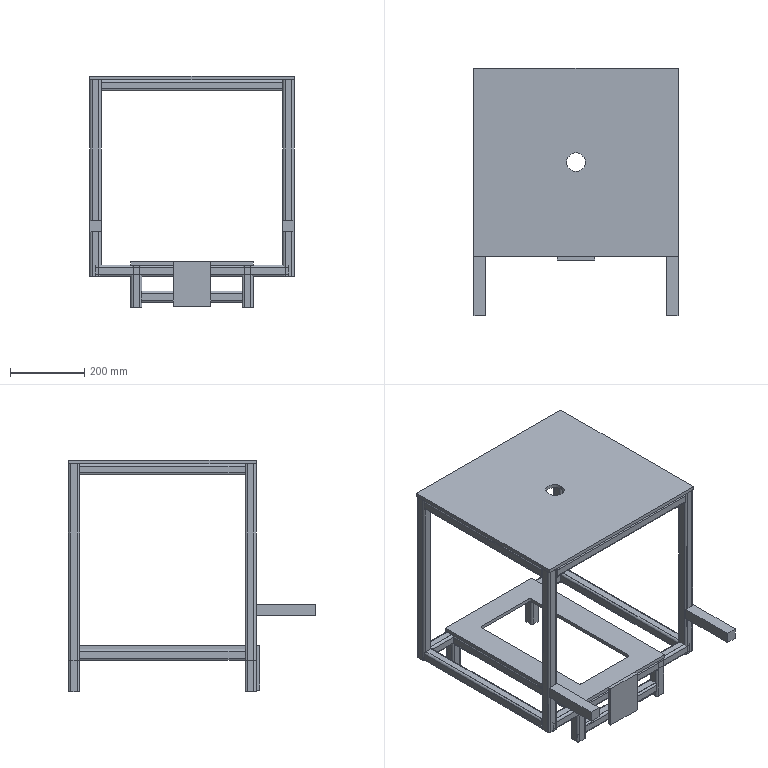Part | STEP file | MYT-A01-P14(Default_machined_) | 28 solids | 422 faces | box 550 x 666 x 625 mm | volume 6400187 mm3 | plane 248 | cylinder 174 | commonest cylinder face diameters 6 x92 12 x76 10 x4 50 x2